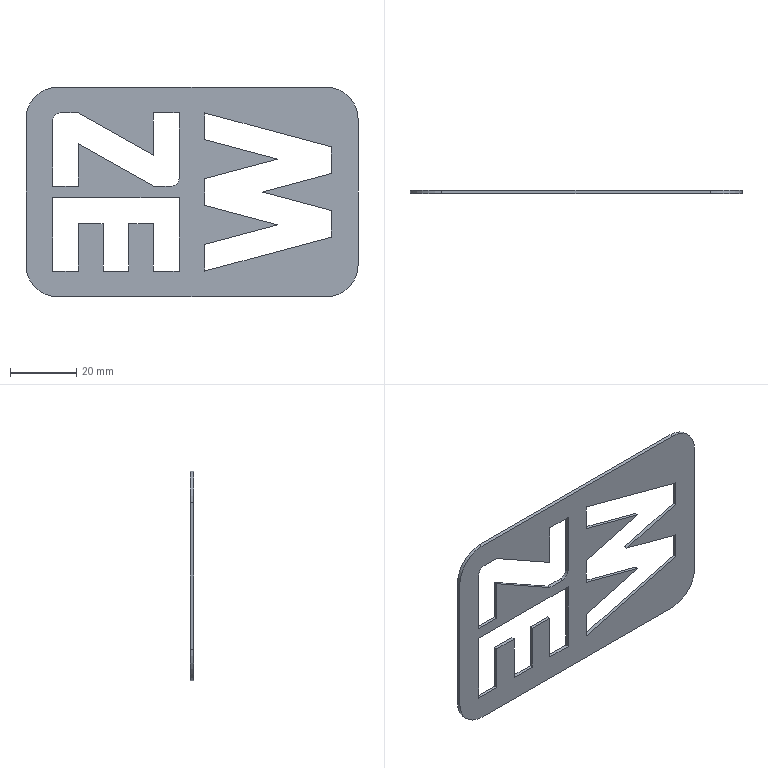Part | STEP file | PRODUCT_ID_96 | 1 solid | 47 faces | box 100 x 1 x 63.1 mm | volume 4008 mm3 | plane 41 | cylinder 6 | commonest cylinder face diameters 19.04 x4 4.76 x2